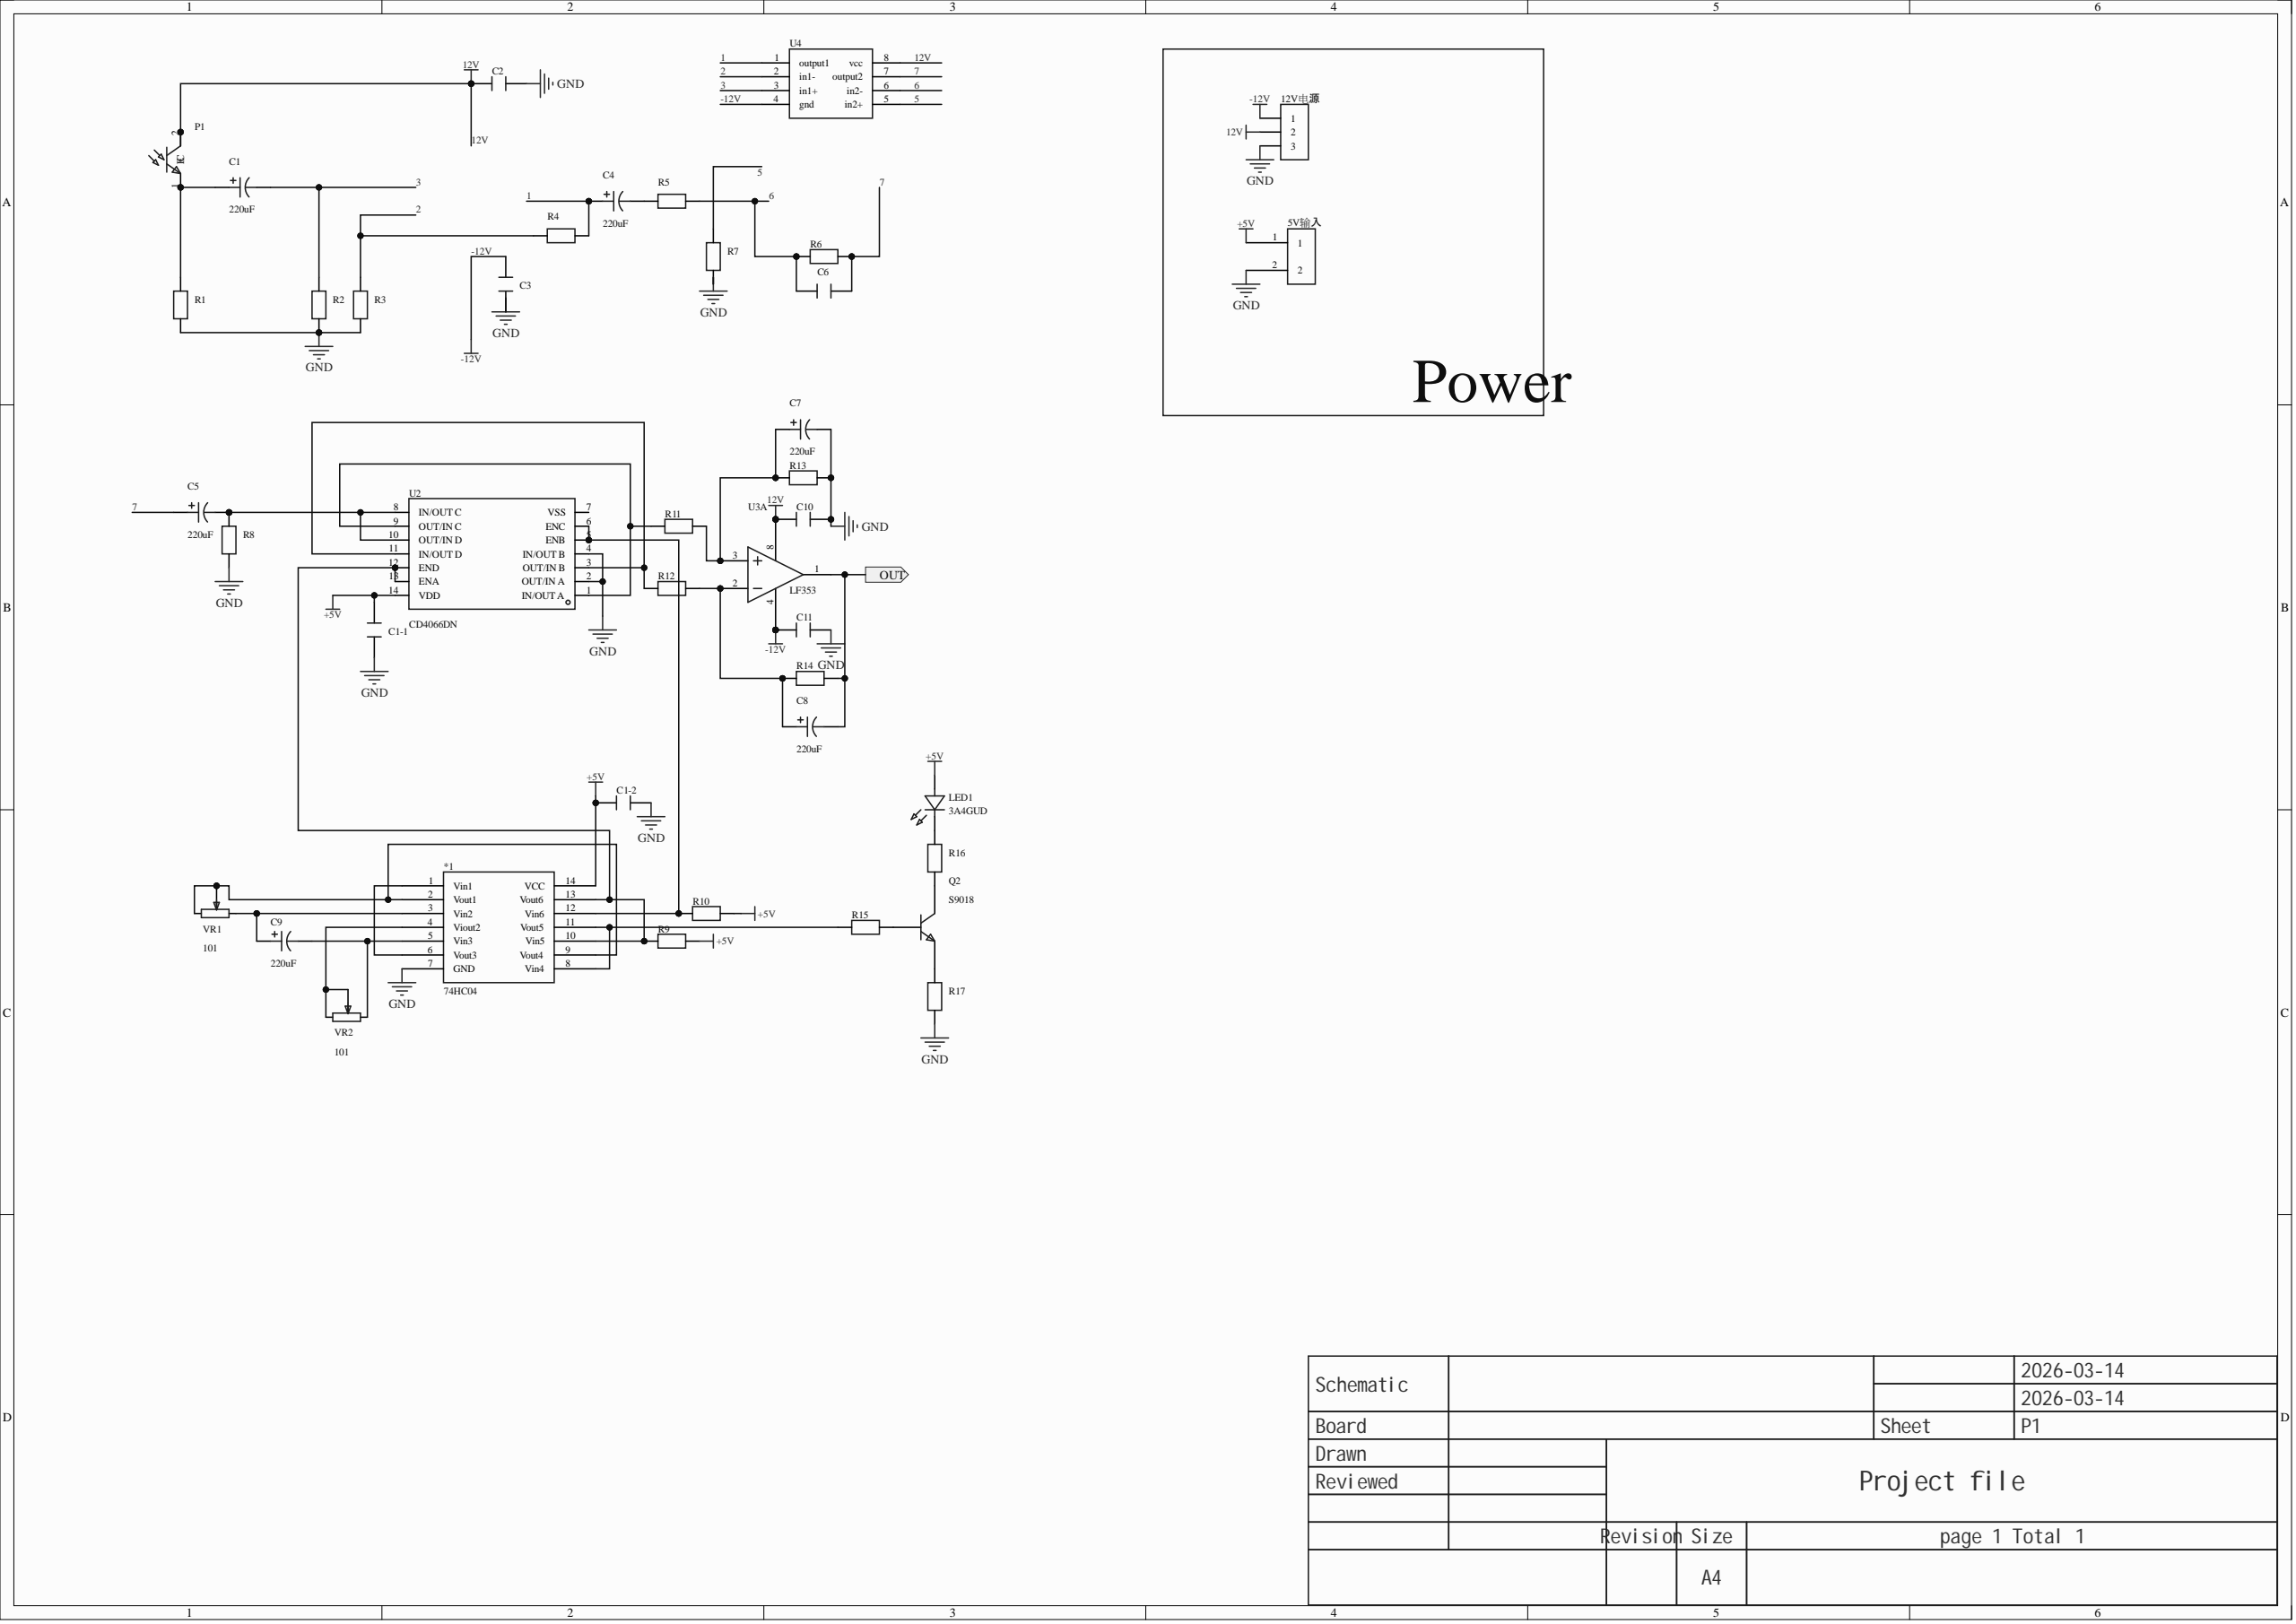Circuit board | Altium Designer | 41 parts | 30 nets
Bill of materials:
Comment,Description,Designator,Footprint,LibRef,Quantity
"74HC04","","*1","DIP14","74HC04","1"
"5V output","","5V输入","2INT","2PIN","1"
"3PIN","","12V电源","3PIN","3PIN","1"
"","","C1-1, C1-2, C2, C3, C6, C10, C11","电容直插","电容直插","7"
"220uF","Capacitance: 220uF; tolerance: ±20%; rated voltage: 16V; ripple current: 300mA@100kHz; equivalent series resistance (ESR): 220mO@100kHz;","C1, C4, C5, C7, C8, C9","CAP-TH_BD6.3-P2.50-D0.5-FD","ERG16V220M6X7","6"
"3A4GUD","Lamp holder type: 3mm round lamp holder; luminous colour: emerald green; forward voltage drop (Vf): 2.8V~3.2V; forward current: 20mA; wavelength: 520nm~525nm; lens colour: green lens; colour temperature: -; luminous intensity: 8000mcd~12000mcd; viewing angle: 30°; operating temperature: -40℃~+85℃;","LED1","LED-TH_BD3.5-P2.54-RD-GREEN","3A4GUD","1"
"","","P1","LED_D3.0mm_Horizontal_O1.27mm_Z2.0mm","LED-3MM-红外接收","1"
"S9018","Transistor type: NPN; collector-emitter breakdown voltage (Vceo): 18V; collector current (Ic): 50mA; power (Pd): 400mW; collector cut-off current (Icbo): 100nA; collector-emitter saturation voltage (VCE(sat)@Ic,Ib): 500mV@10mA,1mA; DC current gain (hFE@Ic,Vce): 97@1mA,5V; transition frequency (fT): 800MHz; operating temperature: +150℃@(Tj);","Q2","TO-92-3_L4.9-W3.7-P1.27-L","S9018","1"
"","Through-hole resistor","R1, R2, R3, R4, R5, R6, R7, R8, R9, R10, R11, R12, R13, R14, R15, R16, R17","D45-V(直插)","直插电阻","17"
"CD4066DN","Switch circuit: 1:1; channels: 4; on-resistance (Ron): 125O;","U2","PDIP-14_L19.3-W6.5-P2.54-LS7.6-BL","CD4066DN","1"
"LF353","","U3","DIP-8","LF353","1"
"","","U4","DIP-8_L9.9-W6.4-P2.54-LS7.6-BL","lf353","1"
"101","","VR1, VR2","3296W","3296","2"
Netlist (Protel format):
[
5V输入
2INT
5V output



]
[
12V电源
3PIN
3PIN



]
[
*1
DIP14
74HC04



]
[
C1
CAP-TH_BD6.3-P2.50-D0.5-FD
220uF



]
[
C1-1
电容直插




]
[
C1-2
电容直插




]
[
C2
电容直插




]
[
C3
电容直插




]
[
C4
CAP-TH_BD6.3-P2.50-D0.5-FD
220uF



]
[
C5
CAP-TH_BD6.3-P2.50-D0.5-FD
220uF



]
[
C6
电容直插




]
[
C7
CAP-TH_BD6.3-P2.50-D0.5-FD
220uF



]
[
C8
CAP-TH_BD6.3-P2.50-D0.5-FD
220uF



]
[
C9
CAP-TH_BD6.3-P2.50-D0.5-FD
220uF



]
[
C10
电容直插




]
[
C11
电容直插




]
[
LED1
LED-TH_BD3.5-P2.54-RD-GREEN
3A4GUD



]
[
P1
LED_D3.0mm_Horizontal_O1.27mm_Z2.0mm




]
[
Q2
TO-92-3_L4.9-W3.7-P1.27-L
S9018



]
[
R1
D45-V(直插)




]
[
R2
D45-V(直插)




]
[
R3
D45-V(直插)




]
[
R4
D45-V(直插)




]
[
R5
D45-V(直插)




]
[
R6
D45-V(直插)




]
[
R7
D45-V(直插)




]
[
R8
D45-V(直插)




]
[
R9
D45-V(直插)




]
[
R10
D45-V(直插)




]
[
R11
D45-V(直插)




]
[
R12
D45-V(直插)




]
[
R13
D45-V(直插)




]
[
R14
D45-V(直插)




]
[
R15
D45-V(直插)




]
[
R16
D45-V(直插)




]
[
R17
D45-V(直插)




]
[
U2
PDIP-14_L19.3-W6.5-P2.54-LS7.6-BL
CD4066DN



]
[
U3
DIP-8
LF353



]
[
U4
DIP-8_L9.9-W6.4-P2.54-LS7.6-BL




]
[
VR1
3296W
101



]
[
VR2
3296W
101



]
(
NetR12_1
R12-1
U2-3
U2-11
)
(
NetR11_1
R11-1
U2-1
U2-9
)
(
NetQ2_3
Q2-3
R16-1
)
(
NetQ2_2
Q2-2
R15-2
)
(
NetQ2_1
Q2-1
R17-2
)
(
NetLED1_1
LED1-1
R16-2
)
(
NetC8_2
C8-2
R14-2
U3-1
)
(
NetC8_1
C8-1
R12-2
R14-1
U3-2
)
(
NetC7_1
C7-1
R11-2
R13-1
U3-3
)
(
NetC5_2
C5-2
R8-1
U2-8
U2-10
)
(
NetC4_2
C4-2
R5-2
)
(
NetC1_1
C1-1
P1-1
R1-1
)
(
Net*1_12
*1-12
R10-1
U2-5
U2-6
)
(
Net*1_10
*1-10
*1-13
R9-1
U2-12
U2-13
)
(
Net*1_8
*1-8
*1-11
R15-1
)
(
Net*1_5
*1-5
C9-2
VR2-3
)
(
Net*1_4
*1-4
VR2-1
VR2-2
)
(
Net*1_3
*1-3
C9-1
VR1-3
)
(
Net*1_2
*1-2
*1-9
VR1-1
VR1-2
)
(
Net*1_1
*1-1
*1-6
)
(
GND
5V输入-2
12V电源-3
*1-7
C1-1-1
C1-2-1
C2-1
C3-1
C7-2
C10-1
C11-1
R1-2
R2-2
R3-2
R7-1
R8-2
R13-2
R17-1
U2-2
U2-4
)
(
-12V
12V电源-1
C3-2
C11-2
U3-4
U4-4
)
(
+5V
5V输入-1
*1-14
C1-1-2
C1-2-2
LED1-2
R9-2
R10-2
U2-14
)
(
12V
12V电源-2
C2-2
C10-2
P1-2
U3-8
U4-8
)
(
7
C5-1
C6-1
R6-2
U4-7
)
(
6
C6-2
R5-1
R6-1
U4-6
)
(
5
R7-2
U4-5
)
(
3
C1-2
R2-1
U4-3
)
(
2
R3-1
R4-2
U4-2
)
(
1
C4-1
R4-1
U4-1
)